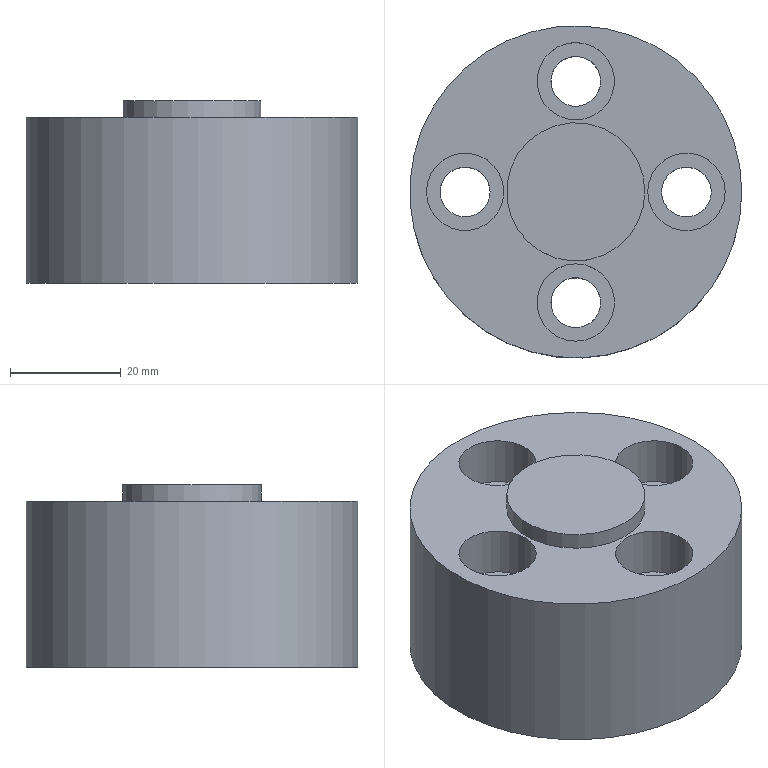CAM job | NX | 3-axis milling, drilling | part box 60 x 60 x 33 mm | stock box 60 x 60 x 33 mm
Tools:
number,name,description,diameter,corner_radius,flute_length,length,flutes
1,D6A45,Milling Tool-5 Parameters,6.0,0.0,50.0,75.0,2
2,9.0ZT,Drilling Tool,9.0,0.0,35.0,50.0,2
10,D10,Milling Tool-5 Parameters,10.0,0.0,50.0,75.0,2
5,ZXZ,Milling Tool-5 Parameters,6.0,0.0,50.0,75.0,2
Operations:
program,operation,operation_type,tool,method,geometry_group,spindle_rpm,surface_speed,feed_per_tooth,feed_cut,feed_plunge,cut_length_mm,path_length_mm,cut_time_min,machine_time_min
1,DRILLING,Operation,ZXZ,METHOD,A,3000.0,0.0,0.0,250.0,0.0,16.0,192.329,0.064,0.0816
1,DRILLING_COPY,Operation,9.0ZT,METHOD,A,1000.0,32.0,0.05,100.0,0.0,144.815,449.96,1.448,1.479
1,HOLE_MILLING,CylinderMilling,D10,METHOD,A,3500.0,109.0,0.3143,2200.0,100.0,2246.286,2629.139,1.021,1.059
1,PLANAR_MILL,PlanarMilling,D6A45,METHOD,A,7500.0,141.0,0.0833,1250.0,100.0,150.443,498.514,0.1204,0.1552